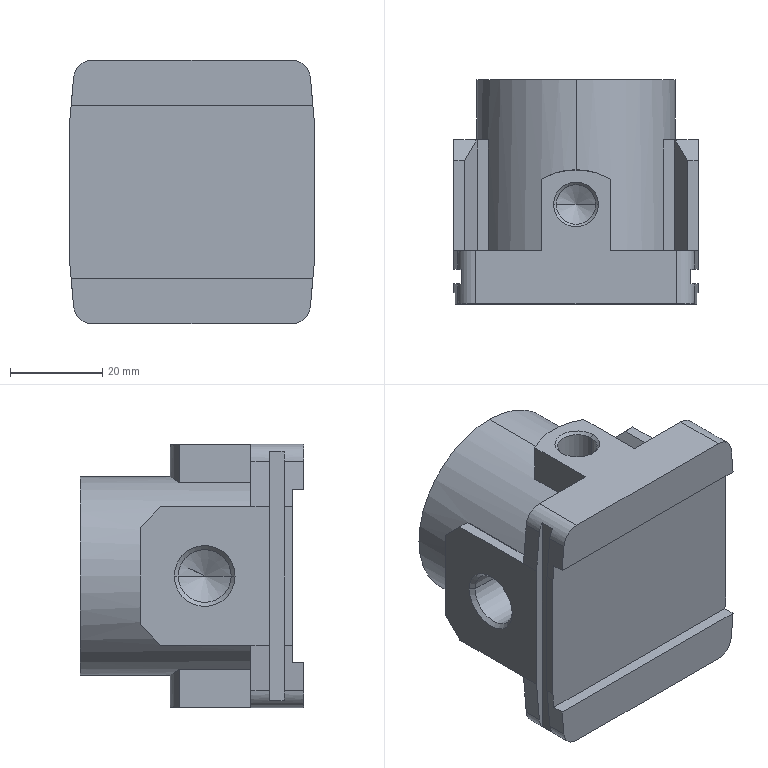Part | STEP file | _AR30-02G-A(0)_BODY | 1 solid | 108 faces | box 53 x 48.5 x 57 mm | volume 90348 mm3 | plane 70 | cylinder 24 | cone 14 | commonest cylinder face diameters 8 x4 11.445 x4 36.4 x3 36.8 x3 8.566 x2 8.6 x2